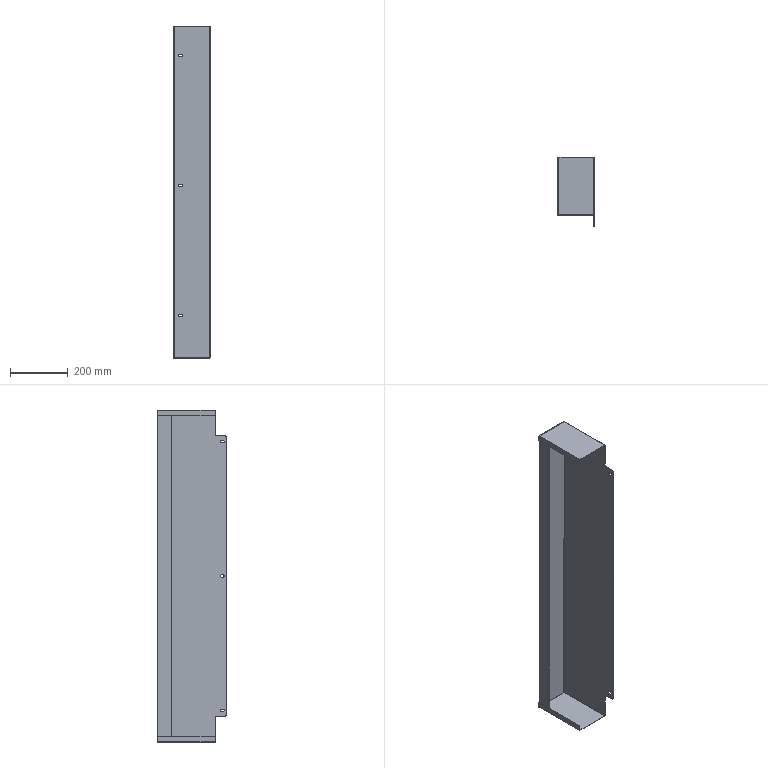Part | SolidWorks | features BaseBody 1 | 1 solid | 107 faces | box 125 x 240 x 1150 mm | volume 623954 mm3 | plane 74 | cylinder 29 | spline 4 | commonest cylinder face diameters 7 x15 1 x6 3.4 x6 10 x2